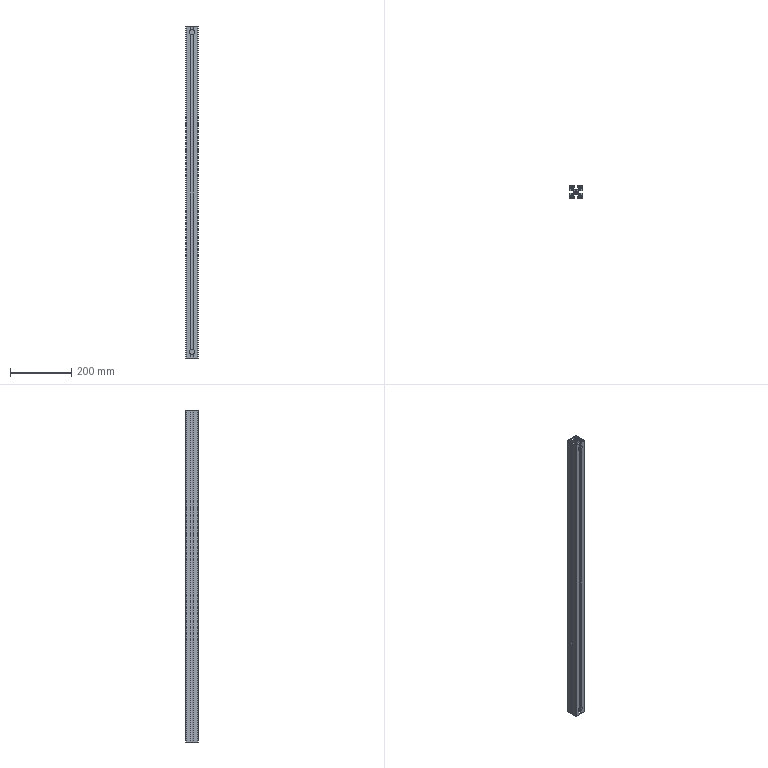Part | STEP file | 09-10 aluminium profile 4040-1080 | 1 solid | 93 faces | box 40 x 40 x 1080 mm | volume 758483 mm3 | plane 62 | cylinder 31 | commonest cylinder face diameters 19 x9 8 x8 18.5 x8 2 x4 6.8 x2